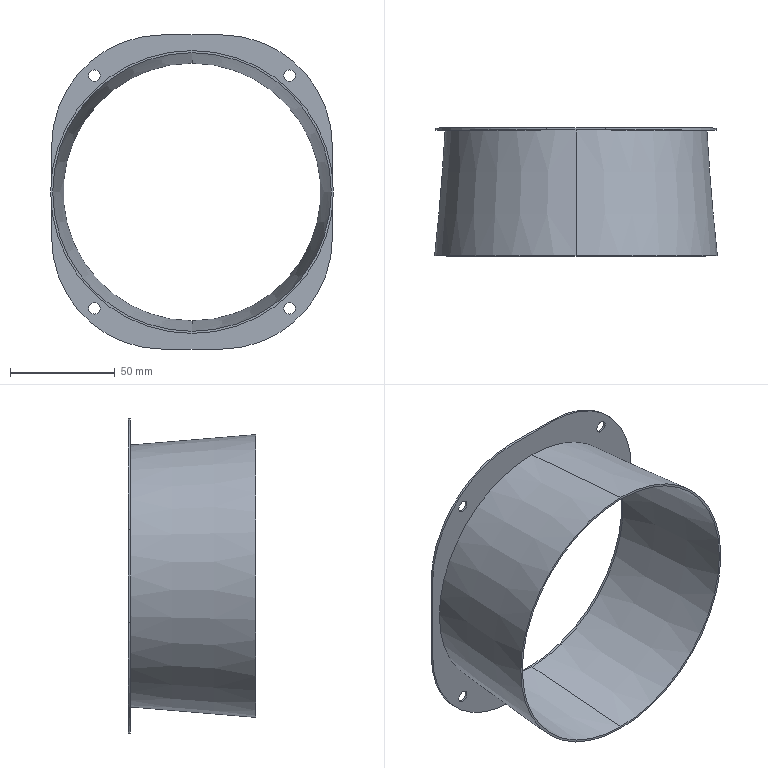Part | SolidWorks | features BaseBody 2 | 2 solids | 26 faces | box 135 x 61 x 150 mm | volume 30112 mm3 | cylinder 14 | plane 8 | cone 4 | commonest cylinder face diameters 5.5 x8 106 x4 122.993 x2
STEP:
#1=CARTESIAN_POINT('',(0.,0.,61.497));
#2=VERTEX_POINT('',#1);
#3=CARTESIAN_POINT('',(0.,-60.,66.497));
#4=VERTEX_POINT('',#3);
#5=CARTESIAN_POINT('',(0.,-0.08305,61.503));
#6=DIRECTION('',(0.,-0.9965,0.08305));
#7=VECTOR('',#6,1000.);
#8=LINE('',#5,#7);
#9=EDGE_CURVE('',#2,#4,#8,.T.);
#10=ORIENTED_EDGE('',*,*,#9,.F.);
#11=CARTESIAN_POINT('',(0.,0.,-61.497));
#12=VERTEX_POINT('',#11);
#13=CARTESIAN_POINT('',(0.,0.,0.));
#14=DIRECTION('',(0.,1.,0.));
#15=DIRECTION('',(0.,0.,1.));
#16=AXIS2_PLACEMENT_3D('',#13,#14,#15);
#17=CIRCLE('',#16,61.497);
#18=EDGE_CURVE('',#2,#12,#17,.T.);
#19=ORIENTED_EDGE('',*,*,#18,.T.);
#20=CARTESIAN_POINT('',(0.,-60.,-66.497));
#21=VERTEX_POINT('',#20);
#22=CARTESIAN_POINT('',(0.,-0.08305,-61.503));
#23=DIRECTION('',(0.,-0.9965,-0.08305));
#24=VECTOR('',#23,1000.);
#25=LINE('',#22,#24);
#26=EDGE_CURVE('',#12,#21,#25,.T.);
#27=ORIENTED_EDGE('',*,*,#26,.T.);
#28=CARTESIAN_POINT('',(0.,-60.,0.));
#29=DIRECTION('',(0.,1.,0.));
#30=DIRECTION('',(0.,0.,1.));
#31=AXIS2_PLACEMENT_3D('',#28,#29,#30);
#32=CIRCLE('',#31,66.497);
#33=EDGE_CURVE('',#4,#21,#32,.T.);
#34=ORIENTED_EDGE('',*,*,#33,.F.);
#35=EDGE_LOOP('',(#10,#19,#27,#34));
#36=FACE_OUTER_BOUND('',#35,.T.);
#37=CARTESIAN_POINT('',(0.,-0.08305,0.));
#38=DIRECTION('',(0.,-1.,0.));
#39=DIRECTION('',(0.,0.,-1.));
#40=AXIS2_PLACEMENT_3D('',#37,#38,#39);
#41=CONICAL_SURFACE('',#40,61.503,0.08314);
#42=ADVANCED_FACE('',(#36),#41,.F.);
#43=CARTESIAN_POINT('',(0.,0.,62.5));
#44=VERTEX_POINT('',#43);
#45=CARTESIAN_POINT('',(0.,-60.,67.5));
#46=VERTEX_POINT('',#45);
#47=CARTESIAN_POINT('',(0.,0.,62.5));
#48=DIRECTION('',(0.,-0.9965,0.08305));
#49=VECTOR('',#48,1000.);
#50=LINE('',#47,#49);
#51=EDGE_CURVE('',#44,#46,#50,.T.);
#52=ORIENTED_EDGE('',*,*,#51,.F.);
#53=CARTESIAN_POINT('',(0.,0.,-62.5));
#54=VERTEX_POINT('',#53);
#55=CARTESIAN_POINT('',(0.,0.,0.));
#56=DIRECTION('',(0.,1.,0.));
#57=DIRECTION('',(0.,0.,1.));
#58=AXIS2_PLACEMENT_3D('',#55,#56,#57);
#59=CIRCLE('',#58,62.5);
#60=EDGE_CURVE('',#54,#44,#59,.T.);
#61=ORIENTED_EDGE('',*,*,#60,.F.);
#62=CARTESIAN_POINT('',(0.,-60.,-67.5));
#63=VERTEX_POINT('',#62);
#64=CARTESIAN_POINT('',(0.,0.,-62.5));
#65=DIRECTION('',(0.,-0.9965,-0.08305));
#66=VECTOR('',#65,1000.);
#67=LINE('',#64,#66);
#68=EDGE_CURVE('',#54,#63,#67,.T.);
#69=ORIENTED_EDGE('',*,*,#68,.T.);
#70=CARTESIAN_POINT('',(0.,-60.,0.));
#71=DIRECTION('',(0.,1.,0.));
#72=DIRECTION('',(0.,0.,1.));
#73=AXIS2_PLACEMENT_3D('',#70,#71,#72);
#74=CIRCLE('',#73,67.5);
#75=EDGE_CURVE('',#63,#46,#74,.T.);
#76=ORIENTED_EDGE('',*,*,#75,.T.);
#77=EDGE_LOOP('',(#52,#61,#69,#76));
#78=FACE_OUTER_BOUND('',#77,.T.);
#79=CARTESIAN_POINT('',(0.,0.,0.));
#80=DIRECTION('',(0.,-1.,0.));
#81=DIRECTION('',(0.,0.,-1.));
#82=AXIS2_PLACEMENT_3D('',#79,#80,#81);
#83=CONICAL_SURFACE('',#82,62.5,0.08314);
#84=ADVANCED_FACE('',(#78),#83,.T.);
#85=CARTESIAN_POINT('',(0.,0.,0.));
#86=DIRECTION('',(0.,1.,0.));
#87=DIRECTION('',(0.,0.,1.));
#88=AXIS2_PLACEMENT_3D('',#85,#86,#87);
#89=CIRCLE('',#88,61.497);
#90=EDGE_CURVE('',#12,#2,#89,.T.);
#91=ORIENTED_EDGE('',*,*,#90,.F.);
#92=ORIENTED_EDGE('',*,*,#18,.F.);
#93=EDGE_LOOP('',(#91,#92));
#94=FACE_BOUND('',#93,.T.);
#95=ORIENTED_EDGE('',*,*,#60,.T.);
#96=CARTESIAN_POINT('',(0.,0.,0.));
#97=DIRECTION('',(0.,1.,0.));
#98=DIRECTION('',(0.,0.,1.));
#99=AXIS2_PLACEMENT_3D('',#96,#97,#98);
#100=CIRCLE('',#99,62.5);
#101=EDGE_CURVE('',#44,#54,#100,.T.);
#102=ORIENTED_EDGE('',*,*,#101,.T.);
#103=EDGE_LOOP('',(#95,#102));
#104=FACE_OUTER_BOUND('',#103,.T.);
#105=CARTESIAN_POINT('',(0.,0.,0.));
#106=DIRECTION('',(0.,1.,0.));
#107=DIRECTION('',(1.,0.,0.));
#108=AXIS2_PLACEMENT_3D('',#105,#106,#107);
#109=PLANE('',#108);
#110=ADVANCED_FACE('',(#94,#104),#109,.T.);
#111=CARTESIAN_POINT('',(0.,-60.,0.));
#112=DIRECTION('',(0.,1.,0.));
#113=DIRECTION('',(0.,0.,1.));
#114=AXIS2_PLACEMENT_3D('',#111,#112,#113);
#115=CIRCLE('',#114,66.497);
#116=EDGE_CURVE('',#21,#4,#115,.T.);
#117=ORIENTED_EDGE('',*,*,#116,.T.);
#118=ORIENTED_EDGE('',*,*,#33,.T.);
#119=EDGE_LOOP('',(#117,#118));
#120=FACE_BOUND('',#119,.T.);
#121=ORIENTED_EDGE('',*,*,#75,.F.);
#122=CARTESIAN_POINT('',(0.,-60.,0.));
#123=DIRECTION('',(0.,1.,0.));
#124=DIRECTION('',(0.,0.,1.));
#125=AXIS2_PLACEMENT_3D('',#122,#123,#124);
#126=CIRCLE('',#125,67.5);
#127=EDGE_CURVE('',#46,#63,#126,.T.);
#128=ORIENTED_EDGE('',*,*,#127,.F.);
#129=EDGE_LOOP('',(#121,#128));
#130=FACE_OUTER_BOUND('',#129,.T.);
#131=CARTESIAN_POINT('',(0.,-60.,0.));
#132=DIRECTION('',(0.,1.,0.));
#133=DIRECTION('',(1.,0.,0.));
#134=AXIS2_PLACEMENT_3D('',#131,#132,#133);
#135=PLANE('',#134);
#136=ADVANCED_FACE('',(#120,#130),#135,.F.);
#137=ORIENTED_EDGE('',*,*,#101,.F.);
#138=ORIENTED_EDGE('',*,*,#51,.T.);
#139=ORIENTED_EDGE('',*,*,#127,.T.);
#140=ORIENTED_EDGE('',*,*,#68,.F.);
#141=EDGE_LOOP('',(#137,#138,#139,#140));
#142=FACE_OUTER_BOUND('',#141,.T.);
#143=CARTESIAN_POINT('',(0.,0.,0.));
#144=DIRECTION('',(0.,-1.,0.));
#145=DIRECTION('',(0.,0.,-1.));
#146=AXIS2_PLACEMENT_3D('',#143,#144,#145);
#147=CONICAL_SURFACE('',#146,62.5,0.08314);
#148=ADVANCED_FACE('',(#142),#147,.T.);
#149=ORIENTED_EDGE('',*,*,#90,.T.);
#150=ORIENTED_EDGE('',*,*,#9,.T.);
#151=ORIENTED_EDGE('',*,*,#116,.F.);
#152=ORIENTED_EDGE('',*,*,#26,.F.);
#153=EDGE_LOOP('',(#149,#150,#151,#152));
#154=FACE_OUTER_BOUND('',#153,.T.);
#155=CARTESIAN_POINT('',(0.,-0.08305,0.));
#156=DIRECTION('',(0.,-1.,0.));
#157=DIRECTION('',(0.,0.,-1.));
#158=AXIS2_PLACEMENT_3D('',#155,#156,#157);
#159=CONICAL_SURFACE('',#158,61.503,0.08314);
#160=ADVANCED_FACE('',(#154),#159,.F.);
#161=CLOSED_SHELL('',(#42,#84,#110,#136,#148,#160));
#162=MANIFOLD_SOLID_BREP('',#161);
#163=CARTESIAN_POINT('',(0.,1.,61.497));
#164=VERTEX_POINT('',#163);
#165=CARTESIAN_POINT('',(0.,0.,61.497));
#166=VERTEX_POINT('',#165);
#167=CARTESIAN_POINT('',(0.,174.938,61.497));
#168=DIRECTION('',(0.,-1.,0.));
#169=VECTOR('',#168,1000.);
#170=LINE('',#167,#169);
#171=EDGE_CURVE('',#164,#166,#170,.T.);
#172=ORIENTED_EDGE('',*,*,#171,.F.);
#173=CARTESIAN_POINT('',(0.,1.,-61.497));
#174=VERTEX_POINT('',#173);
#175=CARTESIAN_POINT('',(0.,1.,0.));
#176=DIRECTION('',(0.,-1.,0.));
#177=DIRECTION('',(0.,0.,1.));
#178=AXIS2_PLACEMENT_3D('',#175,#176,#177);
#179=CIRCLE('',#178,61.497);
#180=EDGE_CURVE('',#174,#164,#179,.T.);
#181=ORIENTED_EDGE('',*,*,#180,.F.);
#182=CARTESIAN_POINT('',(0.,0.,-61.497));
#183=VERTEX_POINT('',#182);
#184=CARTESIAN_POINT('',(0.,174.938,-61.497));
#185=DIRECTION('',(0.,-1.,0.));
#186=VECTOR('',#185,1000.);
#187=LINE('',#184,#186);
#188=EDGE_CURVE('',#174,#183,#187,.T.);
#189=ORIENTED_EDGE('',*,*,#188,.T.);
#190=CARTESIAN_POINT('',(0.,0.,0.));
#191=DIRECTION('',(0.,-1.,0.));
#192=DIRECTION('',(0.,0.,-1.));
#193=AXIS2_PLACEMENT_3D('',#190,#191,#192);
#194=CIRCLE('',#193,61.497);
#195=EDGE_CURVE('',#183,#166,#194,.T.);
#196=ORIENTED_EDGE('',*,*,#195,.T.);
#197=EDGE_LOOP('',(#172,#181,#189,#196));
#198=FACE_OUTER_BOUND('',#197,.T.);
#199=CARTESIAN_POINT('',(0.,174.938,0.));
#200=DIRECTION('',(0.,-1.,0.));
#201=DIRECTION('',(0.,0.,-1.));
#202=AXIS2_PLACEMENT_3D('',#199,#200,#201);
#203=CYLINDRICAL_SURFACE('',#202,61.497);
#204=ADVANCED_FACE('',(#198),#203,.F.);
#205=CARTESIAN_POINT('',(46.602,0.,-58.288));
#206=VERTEX_POINT('',#205);
#207=CARTESIAN_POINT('',(46.602,1.,-58.288));
#208=VERTEX_POINT('',#207);
#209=CARTESIAN_POINT('',(46.602,1.,-58.288));
#210=DIRECTION('',(0.,1.,0.));
#211=VECTOR('',#210,1000.);
#212=LINE('',#209,#211);
#213=EDGE_CURVE('',#206,#208,#212,.T.);
#214=ORIENTED_EDGE('',*,*,#213,.F.);
#215=CARTESIAN_POINT('',(46.602,0.,-52.788));
#216=VERTEX_POINT('',#215);
#217=CARTESIAN_POINT('',(46.602,0.,-55.538));
#218=DIRECTION('',(0.,1.,0.));
#219=DIRECTION('',(0.,0.,1.));
#220=AXIS2_PLACEMENT_3D('',#217,#218,#219);
#221=CIRCLE('',#220,2.75);
#222=EDGE_CURVE('',#216,#206,#221,.T.);
#223=ORIENTED_EDGE('',*,*,#222,.F.);
#224=CARTESIAN_POINT('',(46.602,1.,-52.788));
#225=VERTEX_POINT('',#224);
#226=CARTESIAN_POINT('',(46.602,1.,-52.788));
#227=DIRECTION('',(0.,1.,0.));
#228=VECTOR('',#227,1000.);
#229=LINE('',#226,#228);
#230=EDGE_CURVE('',#216,#225,#229,.T.);
#231=ORIENTED_EDGE('',*,*,#230,.T.);
#232=CARTESIAN_POINT('',(46.602,1.,-55.538));
#233=DIRECTION('',(0.,1.,0.));
#234=DIRECTION('',(0.,0.,1.));
#235=AXIS2_PLACEMENT_3D('',#232,#233,#234);
#236=CIRCLE('',#235,2.75);
#237=EDGE_CURVE('',#225,#208,#236,.T.);
#238=ORIENTED_EDGE('',*,*,#237,.T.);
#239=EDGE_LOOP('',(#214,#223,#231,#238));
#240=FACE_OUTER_BOUND('',#239,.T.);
#241=CARTESIAN_POINT('',(46.602,1.,-55.538));
#242=DIRECTION('',(0.,1.,0.));
#243=DIRECTION('',(0.,0.,1.));
#244=AXIS2_PLACEMENT_3D('',#241,#242,#243);
#245=CYLINDRICAL_SURFACE('',#244,2.75);
#246=ADVANCED_FACE('',(#240),#245,.F.);
#247=CARTESIAN_POINT('',(46.602,0.,52.788));
#248=VERTEX_POINT('',#247);
#249=CARTESIAN_POINT('',(46.602,1.,52.788));
#250=VERTEX_POINT('',#249);
#251=CARTESIAN_POINT('',(46.602,1.,52.788));
#252=DIRECTION('',(0.,1.,0.));
#253=VECTOR('',#252,1000.);
#254=LINE('',#251,#253);
#255=EDGE_CURVE('',#248,#250,#254,.T.);
#256=ORIENTED_EDGE('',*,*,#255,.F.);
#257=CARTESIAN_POINT('',(46.602,0.,58.288));
#258=VERTEX_POINT('',#257);
#259=CARTESIAN_POINT('',(46.602,0.,55.538));
#260=DIRECTION('',(0.,1.,0.));
#261=DIRECTION('',(0.,0.,1.));
#262=AXIS2_PLACEMENT_3D('',#259,#260,#261);
#263=CIRCLE('',#262,2.75);
#264=EDGE_CURVE('',#258,#248,#263,.T.);
#265=ORIENTED_EDGE('',*,*,#264,.F.);
#266=CARTESIAN_POINT('',(46.602,1.,58.288));
#267=VERTEX_POINT('',#266);
#268=CARTESIAN_POINT('',(46.602,1.,58.288));
#269=DIRECTION('',(0.,1.,0.));
#270=VECTOR('',#269,1000.);
#271=LINE('',#268,#270);
#272=EDGE_CURVE('',#258,#267,#271,.T.);
#273=ORIENTED_EDGE('',*,*,#272,.T.);
#274=CARTESIAN_POINT('',(46.602,1.,55.538));
#275=DIRECTION('',(0.,1.,0.));
#276=DIRECTION('',(0.,0.,1.));
#277=AXIS2_PLACEMENT_3D('',#274,#275,#276);
#278=CIRCLE('',#277,2.75);
#279=EDGE_CURVE('',#267,#250,#278,.T.);
#280=ORIENTED_EDGE('',*,*,#279,.T.);
#281=EDGE_LOOP('',(#256,#265,#273,#280));
#282=FACE_OUTER_BOUND('',#281,.T.);
#283=CARTESIAN_POINT('',(46.602,1.,55.538));
#284=DIRECTION('',(0.,1.,0.));
#285=DIRECTION('',(0.,0.,1.));
#286=AXIS2_PLACEMENT_3D('',#283,#284,#285);
#287=CYLINDRICAL_SURFACE('',#286,2.75);
#288=ADVANCED_FACE('',(#282),#287,.F.);
#289=CARTESIAN_POINT('',(-46.602,0.,52.788));
#290=VERTEX_POINT('',#289);
#291=CARTESIAN_POINT('',(-46.602,1.,52.788));
#292=VERTEX_POINT('',#291);
#293=CARTESIAN_POINT('',(-46.602,1.,52.788));
#294=DIRECTION('',(0.,1.,0.));
#295=VECTOR('',#294,1000.);
#296=LINE('',#293,#295);
#297=EDGE_CURVE('',#290,#292,#296,.T.);
#298=ORIENTED_EDGE('',*,*,#297,.F.);
#299=CARTESIAN_POINT('',(-46.602,0.,58.288));
#300=VERTEX_POINT('',#299);
#301=CARTESIAN_POINT('',(-46.602,0.,55.538));
#302=DIRECTION('',(0.,1.,0.));
#303=DIRECTION('',(0.,0.,1.));
#304=AXIS2_PLACEMENT_3D('',#301,#302,#303);
#305=CIRCLE('',#304,2.75);
#306=EDGE_CURVE('',#300,#290,#305,.T.);
#307=ORIENTED_EDGE('',*,*,#306,.F.);
#308=CARTESIAN_POINT('',(-46.602,1.,58.288));
#309=VERTEX_POINT('',#308);
#310=CARTESIAN_POINT('',(-46.602,1.,58.288));
#311=DIRECTION('',(0.,1.,0.));
#312=VECTOR('',#311,1000.);
#313=LINE('',#310,#312);
#314=EDGE_CURVE('',#300,#309,#313,.T.);
#315=ORIENTED_EDGE('',*,*,#314,.T.);
#316=CARTESIAN_POINT('',(-46.602,1.,55.538));
#317=DIRECTION('',(0.,1.,0.));
#318=DIRECTION('',(0.,0.,1.));
#319=AXIS2_PLACEMENT_3D('',#316,#317,#318);
#320=CIRCLE('',#319,2.75);
#321=EDGE_CURVE('',#309,#292,#320,.T.);
#322=ORIENTED_EDGE('',*,*,#321,.T.);
#323=EDGE_LOOP('',(#298,#307,#315,#322));
#324=FACE_OUTER_BOUND('',#323,.T.);
#325=CARTESIAN_POINT('',(-46.602,1.,55.538));
#326=DIRECTION('',(0.,1.,0.));
#327=DIRECTION('',(0.,0.,1.));
#328=AXIS2_PLACEMENT_3D('',#325,#326,#327);
#329=CYLINDRICAL_SURFACE('',#328,2.75);
#330=ADVANCED_FACE('',(#324),#329,.F.);
#331=CARTESIAN_POINT('',(-46.602,0.,-58.288));
#332=VERTEX_POINT('',#331);
#333=CARTESIAN_POINT('',(-46.602,1.,-58.288));
#334=VERTEX_POINT('',#333);
#335=CARTESIAN_POINT('',(-46.602,1.,-58.288));
#336=DIRECTION('',(0.,1.,0.));
#337=VECTOR('',#336,1000.);
#338=LINE('',#335,#337);
#339=EDGE_CURVE('',#332,#334,#338,.T.);
#340=ORIENTED_EDGE('',*,*,#339,.F.);
#341=CARTESIAN_POINT('',(-46.602,0.,-52.788));
#342=VERTEX_POINT('',#341);
#343=CARTESIAN_POINT('',(-46.602,0.,-55.538));
#344=DIRECTION('',(0.,1.,0.));
#345=DIRECTION('',(0.,0.,1.));
#346=AXIS2_PLACEMENT_3D('',#343,#344,#345);
#347=CIRCLE('',#346,2.75);
#348=EDGE_CURVE('',#342,#332,#347,.T.);
#349=ORIENTED_EDGE('',*,*,#348,.F.);
#350=CARTESIAN_POINT('',(-46.602,1.,-52.788));
#351=VERTEX_POINT('',#350);
#352=CARTESIAN_POINT('',(-46.602,1.,-52.788));
#353=DIRECTION('',(0.,1.,0.));
#354=VECTOR('',#353,1000.);
#355=LINE('',#352,#354);
#356=EDGE_CURVE('',#342,#351,#355,.T.);
#357=ORIENTED_EDGE('',*,*,#356,.T.);
#358=CARTESIAN_POINT('',(-46.602,1.,-55.538));
#359=DIRECTION('',(0.,1.,0.));
#360=DIRECTION('',(0.,0.,1.));
#361=AXIS2_PLACEMENT_3D('',#358,#359,#360);
#362=CIRCLE('',#361,2.75);
#363=EDGE_CURVE('',#351,#334,#362,.T.);
#364=ORIENTED_EDGE('',*,*,#363,.T.);
#365=EDGE_LOOP('',(#340,#349,#357,#364));
#366=FACE_OUTER_BOUND('',#365,.T.);
#367=CARTESIAN_POINT('',(-46.602,1.,-55.538));
#368=DIRECTION('',(0.,1.,0.));
#369=DIRECTION('',(0.,0.,1.));
#370=AXIS2_PLACEMENT_3D('',#367,#368,#369);
#371=CYLINDRICAL_SURFACE('',#370,2.75);
#372=ADVANCED_FACE('',(#366),#371,.F.);
#373=ORIENTED_EDGE('',*,*,#348,.T.);
#374=CARTESIAN_POINT('',(-46.602,0.,-55.538));
#375=DIRECTION('',(0.,1.,0.));
#376=DIRECTION('',(0.,0.,1.));
#377=AXIS2_PLACEMENT_3D('',#374,#375,#376);
#378=CIRCLE('',#377,2.75);
#379=EDGE_CURVE('',#332,#342,#378,.T.);
#380=ORIENTED_EDGE('',*,*,#379,.T.);
#381=EDGE_LOOP('',(#373,#380));
#382=FACE_BOUND('',#381,.T.);
#383=ORIENTED_EDGE('',*,*,#306,.T.);
#384=CARTESIAN_POINT('',(-46.602,0.,55.538));
#385=DIRECTION('',(0.,1.,0.));
#386=DIRECTION('',(0.,0.,1.));
#387=AXIS2_PLACEMENT_3D('',#384,#385,#386);
#388=CIRCLE('',#387,2.75);
#389=EDGE_CURVE('',#290,#300,#388,.T.);
#390=ORIENTED_EDGE('',*,*,#389,.T.);
#391=EDGE_LOOP('',(#383,#390));
#392=FACE_BOUND('',#391,.T.);
#393=ORIENTED_EDGE('',*,*,#264,.T.);
#394=CARTESIAN_POINT('',(46.602,0.,55.538));
#395=DIRECTION('',(0.,1.,0.));
#396=DIRECTION('',(0.,0.,1.));
#397=AXIS2_PLACEMENT_3D('',#394,#395,#396);
#398=CIRCLE('',#397,2.75);
#399=EDGE_CURVE('',#248,#258,#398,.T.);
#400=ORIENTED_EDGE('',*,*,#399,.T.);
#401=EDGE_LOOP('',(#393,#400));
#402=FACE_BOUND('',#401,.T.);
#403=ORIENTED_EDGE('',*,*,#222,.T.);
#404=CARTESIAN_POINT('',(46.602,0.,-55.538));
#405=DIRECTION('',(0.,1.,0.));
#406=DIRECTION('',(0.,0.,1.));
#407=AXIS2_PLACEMENT_3D('',#404,#405,#406);
#408=CIRCLE('',#407,2.75);
#409=EDGE_CURVE('',#206,#216,#408,.T.);
#410=ORIENTED_EDGE('',*,*,#409,.T.);
#411=EDGE_LOOP('',(#403,#410));
#412=FACE_BOUND('',#411,.T.);
#413=ORIENTED_EDGE('',*,*,#195,.F.);
#414=CARTESIAN_POINT('',(0.,0.,0.));
#415=DIRECTION('',(0.,-1.,0.));
#416=DIRECTION('',(0.,0.,-1.));
#417=AXIS2_PLACEMENT_3D('',#414,#415,#416);
#418=CIRCLE('',#417,61.497);
#419=EDGE_CURVE('',#166,#183,#418,.T.);
#420=ORIENTED_EDGE('',*,*,#419,.F.);
#421=EDGE_LOOP('',(#413,#420));
#422=FACE_BOUND('',#421,.T.);
#423=CARTESIAN_POINT('',(14.,0.,75.));
#424=VERTEX_POINT('',#423);
#425=CARTESIAN_POINT('',(67.,0.,22.));
#426=VERTEX_POINT('',#425);
#427=CARTESIAN_POINT('',(14.,0.,22.));
#428=DIRECTION('',(0.,1.,0.));
#429=DIRECTION('',(0.,0.,1.));
#430=AXIS2_PLACEMENT_3D('',#427,#428,#429);
#431=CIRCLE('',#430,53.);
#432=EDGE_CURVE('',#424,#426,#431,.T.);
#433=ORIENTED_EDGE('',*,*,#432,.F.);
#434=CARTESIAN_POINT('',(-14.,0.,75.));
#435=VERTEX_POINT('',#434);
#436=CARTESIAN_POINT('',(14.,0.,75.));
#437=DIRECTION('',(1.,0.,0.));
#438=VECTOR('',#437,1000.);
#439=LINE('',#436,#438);
#440=EDGE_CURVE('',#435,#424,#439,.T.);
#441=ORIENTED_EDGE('',*,*,#440,.F.);
#442=CARTESIAN_POINT('',(-67.,0.,22.));
#443=VERTEX_POINT('',#442);
#444=CARTESIAN_POINT('',(-14.,0.,22.));
#445=DIRECTION('',(0.,1.,0.));
#446=DIRECTION('',(0.,0.,-1.));
#447=AXIS2_PLACEMENT_3D('',#444,#445,#446);
#448=CIRCLE('',#447,53.);
#449=EDGE_CURVE('',#443,#435,#448,.T.);
#450=ORIENTED_EDGE('',*,*,#449,.F.);
#451=CARTESIAN_POINT('',(-67.,0.,-22.));
#452=VERTEX_POINT('',#451);
#453=CARTESIAN_POINT('',(-67.,0.,22.));
#454=DIRECTION('',(0.,0.,1.));
#455=VECTOR('',#454,1000.);
#456=LINE('',#453,#455);
#457=EDGE_CURVE('',#452,#443,#456,.T.);
#458=ORIENTED_EDGE('',*,*,#457,.F.);
#459=CARTESIAN_POINT('',(-14.,0.,-75.));
#460=VERTEX_POINT('',#459);
#461=CARTESIAN_POINT('',(-14.,0.,-22.));
#462=DIRECTION('',(0.,1.,0.));
#463=DIRECTION('',(0.,0.,1.));
#464=AXIS2_PLACEMENT_3D('',#461,#462,#463);
#465=CIRCLE('',#464,53.);
#466=EDGE_CURVE('',#460,#452,#465,.T.);
#467=ORIENTED_EDGE('',*,*,#466,.F.);
#468=CARTESIAN_POINT('',(14.,0.,-75.));
#469=VERTEX_POINT('',#468);
#470=CARTESIAN_POINT('',(14.,0.,-75.));
#471=DIRECTION('',(-1.,0.,0.));
#472=VECTOR('',#471,1000.);
#473=LINE('',#470,#472);
#474=EDGE_CURVE('',#469,#460,#473,.T.);
#475=ORIENTED_EDGE('',*,*,#474,.F.);
#476=CARTESIAN_POINT('',(67.,0.,-22.));
#477=VERTEX_POINT('',#476);
#478=CARTESIAN_POINT('',(14.,0.,-22.));
#479=DIRECTION('',(0.,1.,0.));
#480=DIRECTION('',(0.,0.,1.));
#481=AXIS2_PLACEMENT_3D('',#478,#479,#480);
#482=CIRCLE('',#481,53.);
#483=EDGE_CURVE('',#477,#469,#482,.T.);
#484=ORIENTED_EDGE('',*,*,#483,.F.);
#485=CARTESIAN_POINT('',(67.,0.,22.));
#486=DIRECTION('',(0.,0.,-1.));
#487=VECTOR('',#486,1000.);
#488=LINE('',#485,#487);
#489=EDGE_CURVE('',#426,#477,#488,.T.);
#490=ORIENTED_EDGE('',*,*,#489,.F.);
#491=EDGE_LOOP('',(#433,#441,#450,#458,#467,#475,#484,#490));
#492=FACE_OUTER_BOUND('',#491,.T.);
#493=CARTESIAN_POINT('',(14.,0.,22.));
#494=DIRECTION('',(0.,1.,0.));
#495=DIRECTION('',(1.,0.,0.));
#496=AXIS2_PLACEMENT_3D('',#493,#494,#495);
#497=PLANE('',#496);
#498=ADVANCED_FACE('',(#382,#392,#402,#412,#422,#492),#497,.F.);
#499=ORIENTED_EDGE('',*,*,#363,.F.);
#500=CARTESIAN_POINT('',(-46.602,1.,-55.538));
#501=DIRECTION('',(0.,1.,0.));
#502=DIRECTION('',(0.,0.,1.));
#503=AXIS2_PLACEMENT_3D('',#500,#501,#502);
#504=CIRCLE('',#503,2.75);
#505=EDGE_CURVE('',#334,#351,#504,.T.);
#506=ORIENTED_EDGE('',*,*,#505,.F.);
#507=EDGE_LOOP('',(#499,#506));
#508=FACE_BOUND('',#507,.T.);
#509=ORIENTED_EDGE('',*,*,#321,.F.);
#510=CARTESIAN_POINT('',(-46.602,1.,55.538));
#511=DIRECTION('',(0.,1.,0.));
#512=DIRECTION('',(0.,0.,1.));
#513=AXIS2_PLACEMENT_3D('',#510,#511,#512);
#514=CIRCLE('',#513,2.75);
#515=EDGE_CURVE('',#292,#309,#514,.T.);
#516=ORIENTED_EDGE('',*,*,#515,.F.);
#517=EDGE_LOOP('',(#509,#516));
#518=FACE_BOUND('',#517,.T.);
#519=ORIENTED_EDGE('',*,*,#279,.F.);
#520=CARTESIAN_POINT('',(46.602,1.,55.538));
#521=DIRECTION('',(0.,1.,0.));
#522=DIRECTION('',(0.,0.,1.));
#523=AXIS2_PLACEMENT_3D('',#520,#521,#522);
#524=CIRCLE('',#523,2.75);
#525=EDGE_CURVE('',#250,#267,#524,.T.);
#526=ORIENTED_EDGE('',*,*,#525,.F.);
#527=EDGE_LOOP('',(#519,#526));
#528=FACE_BOUND('',#527,.T.);
#529=ORIENTED_EDGE('',*,*,#237,.F.);
#530=CARTESIAN_POINT('',(46.602,1.,-55.538));
#531=DIRECTION('',(0.,1.,0.));
#532=DIRECTION('',(0.,0.,1.));
#533=AXIS2_PLACEMENT_3D('',#530,#531,#532);
#534=CIRCLE('',#533,2.75);
#535=EDGE_CURVE('',#208,#225,#534,.T.);
#536=ORIENTED_EDGE('',*,*,#535,.F.);
#537=EDGE_LOOP('',(#529,#536));
#538=FACE_BOUND('',#537,.T.);
#539=ORIENTED_EDGE('',*,*,#180,.T.);
#540=CARTESIAN_POINT('',(0.,1.,0.));
#541=DIRECTION('',(0.,-1.,0.));
#542=DIRECTION('',(0.,0.,1.));
#543=AXIS2_PLACEMENT_3D('',#540,#541,#542);
#544=CIRCLE('',#543,61.497);
#545=EDGE_CURVE('',#164,#174,#544,.T.);
#546=ORIENTED_EDGE('',*,*,#545,.T.);
#547=EDGE_LOOP('',(#539,#546));
#548=FACE_BOUND('',#547,.T.);
#549=CARTESIAN_POINT('',(14.,1.,75.));
#550=VERTEX_POINT('',#549);
#551=CARTESIAN_POINT('',(67.,1.,22.));
#552=VERTEX_POINT('',#551);
#553=CARTESIAN_POINT('',(14.,1.,22.));
#554=DIRECTION('',(0.,1.,0.));
#555=DIRECTION('',(0.,0.,1.));
#556=AXIS2_PLACEMENT_3D('',#553,#554,#555);
#557=CIRCLE('',#556,53.);
#558=EDGE_CURVE('',#550,#552,#557,.T.);
#559=ORIENTED_EDGE('',*,*,#558,.T.);
#560=CARTESIAN_POINT('',(67.,1.,-22.));
#561=VERTEX_POINT('',#560);
#562=CARTESIAN_POINT('',(67.,1.,22.));
#563=DIRECTION('',(0.,0.,-1.));
#564=VECTOR('',#563,1000.);
#565=LINE('',#562,#564);
#566=EDGE_CURVE('',#552,#561,#565,.T.);
#567=ORIENTED_EDGE('',*,*,#566,.T.);
#568=CARTESIAN_POINT('',(14.,1.,-75.));
#569=VERTEX_POINT('',#568);
#570=CARTESIAN_POINT('',(14.,1.,-22.));
#571=DIRECTION('',(0.,1.,0.));
#572=DIRECTION('',(0.,0.,1.));
#573=AXIS2_PLACEMENT_3D('',#570,#571,#572);
#574=CIRCLE('',#573,53.);
#575=EDGE_CURVE('',#561,#569,#574,.T.);
#576=ORIENTED_EDGE('',*,*,#575,.T.);
#577=CARTESIAN_POINT('',(-14.,1.,-75.));
#578=VERTEX_POINT('',#577);
#579=CARTESIAN_POINT('',(14.,1.,-75.));
#580=DIRECTION('',(-1.,0.,0.));
#581=VECTOR('',#580,1000.);
#582=LINE('',#579,#581);
#583=EDGE_CURVE('',#569,#578,#582,.T.);
#584=ORIENTED_EDGE('',*,*,#583,.T.);
#585=CARTESIAN_POINT('',(-67.,1.,-22.));
#586=VERTEX_POINT('',#585);
#587=CARTESIAN_POINT('',(-14.,1.,-22.));
#588=DIRECTION('',(0.,1.,0.));
#589=DIRECTION('',(0.,0.,1.));
#590=AXIS2_PLACEMENT_3D('',#587,#588,#589);
#591=CIRCLE('',#590,53.);
#592=EDGE_CURVE('',#578,#586,#591,.T.);
#593=ORIENTED_EDGE('',*,*,#592,.T.);
#594=CARTESIAN_POINT('',(-67.,1.,22.));
#595=VERTEX_POINT('',#594);
#596=CARTESIAN_POINT('',(-67.,1.,22.));
#597=DIRECTION('',(0.,0.,1.));
#598=VECTOR('',#597,1000.);
#599=LINE('',#596,#598);
#600=EDGE_CURVE('',#586,#595,#599,.T.);
#601=ORIENTED_EDGE('',*,*,#600,.T.);
#602=CARTESIAN_POINT('',(-14.,1.,75.));
#603=VERTEX_POINT('',#602);
#604=CARTESIAN_POINT('',(-14.,1.,22.));
#605=DIRECTION('',(0.,1.,0.));
#606=DIRECTION('',(0.,0.,-1.));
#607=AXIS2_PLACEMENT_3D('',#604,#605,#606);
#608=CIRCLE('',#607,53.);
#609=EDGE_CURVE('',#595,#603,#608,.T.);
#610=ORIENTED_EDGE('',*,*,#609,.T.);
#611=CARTESIAN_POINT('',(14.,1.,75.));
#612=DIRECTION('',(1.,0.,0.));
#613=VECTOR('',#612,1000.);
#614=LINE('',#611,#613);
#615=EDGE_CURVE('',#603,#550,#614,.T.);
#616=ORIENTED_EDGE('',*,*,#615,.T.);
#617=EDGE_LOOP('',(#559,#567,#576,#584,#593,#601,#610,#616));
#618=FACE_OUTER_BOUND('',#617,.T.);
#619=CARTESIAN_POINT('',(14.,1.,22.));
#620=DIRECTION('',(0.,1.,0.));
#621=DIRECTION('',(1.,0.,0.));
#622=AXIS2_PLACEMENT_3D('',#619,#620,#621);
#623=PLANE('',#622);
#624=ADVANCED_FACE('',(#508,#518,#528,#538,#548,#618),#623,.T.);
#625=ORIENTED_EDGE('',*,*,#440,.T.);
#626=CARTESIAN_POINT('',(14.,1.,75.));
#627=DIRECTION('',(0.,-1.,0.));
#628=VECTOR('',#627,1000.);
#629=LINE('',#626,#628);
#630=EDGE_CURVE('',#550,#424,#629,.T.);
#631=ORIENTED_EDGE('',*,*,#630,.F.);
#632=ORIENTED_EDGE('',*,*,#615,.F.);
#633=CARTESIAN_POINT('',(-14.,1.,75.));
#634=DIRECTION('',(0.,-1.,0.));
#635=VECTOR('',#634,1000.);
#636=LINE('',#633,#635);
#637=EDGE_CURVE('',#603,#435,#636,.T.);
#638=ORIENTED_EDGE('',*,*,#637,.T.);
#639=EDGE_LOOP('',(#625,#631,#632,#638));
#640=FACE_OUTER_BOUND('',#639,.T.);
#641=CARTESIAN_POINT('',(14.,1.,75.));
#642=DIRECTION('',(0.,0.,-1.));
#643=DIRECTION('',(0.,-1.,0.));
#644=AXIS2_PLACEMENT_3D('',#641,#642,#643);
#645=PLANE('',#644);
#646=ADVANCED_FACE('',(#640),#645,.F.);
#647=ORIENTED_EDGE('',*,*,#449,.T.);
#648=ORIENTED_EDGE('',*,*,#637,.F.);
#649=ORIENTED_EDGE('',*,*,#609,.F.);
#650=CARTESIAN_POINT('',(-67.,1.,22.));
#651=DIRECTION('',(0.,-1.,0.));
#652=VECTOR('',#651,1000.);
#653=LINE('',#650,#652);
#654=EDGE_CURVE('',#595,#443,#653,.T.);
#655=ORIENTED_EDGE('',*,*,#654,.T.);
#656=EDGE_LOOP('',(#647,#648,#649,#655));
#657=FACE_OUTER_BOUND('',#656,.T.);
#658=CARTESIAN_POINT('',(-14.,1.,22.));
#659=DIRECTION('',(0.,-1.,0.));
#660=DIRECTION('',(0.,0.,-1.));
#661=AXIS2_PLACEMENT_3D('',#658,#659,#660);
#662=CYLINDRICAL_SURFACE('',#661,53.);
#663=ADVANCED_FACE('',(#657),#662,.T.);
#664=ORIENTED_EDGE('',*,*,#457,.T.);
#665=ORIENTED_EDGE('',*,*,#654,.F.);
#666=ORIENTED_EDGE('',*,*,#600,.F.);
#667=CARTESIAN_POINT('',(-67.,1.,-22.));
#668=DIRECTION('',(0.,-1.,0.));
#669=VECTOR('',#668,1000.);
#670=LINE('',#667,#669);
#671=EDGE_CURVE('',#586,#452,#670,.T.);
#672=ORIENTED_EDGE('',*,*,#671,.T.);
#673=EDGE_LOOP('',(#664,#665,#666,#672));
#674=FACE_OUTER_BOUND('',#673,.T.);
#675=CARTESIAN_POINT('',(-67.,1.,22.));
#676=DIRECTION('',(1.,0.,0.));
#677=DIRECTION('',(0.,1.,0.));
#678=AXIS2_PLACEMENT_3D('',#675,#676,#677);
#679=PLANE('',#678);
#680=ADVANCED_FACE('',(#674),#679,.F.);
#681=ORIENTED_EDGE('',*,*,#466,.T.);
#682=ORIENTED_EDGE('',*,*,#671,.F.);
#683=ORIENTED_EDGE('',*,*,#592,.F.);
#684=CARTESIAN_POINT('',(-14.,1.,-75.));
#685=DIRECTION('',(0.,-1.,0.));
#686=VECTOR('',#685,1000.);
#687=LINE('',#684,#686);
#688=EDGE_CURVE('',#578,#460,#687,.T.);
#689=ORIENTED_EDGE('',*,*,#688,.T.);
#690=EDGE_LOOP('',(#681,#682,#683,#689));
#691=FACE_OUTER_BOUND('',#690,.T.);
#692=CARTESIAN_POINT('',(-14.,1.,-22.));
#693=DIRECTION('',(0.,-1.,0.));
#694=DIRECTION('',(0.,0.,-1.));
#695=AXIS2_PLACEMENT_3D('',#692,#693,#694);
#696=CYLINDRICAL_SURFACE('',#695,53.);
#697=ADVANCED_FACE('',(#691),#696,.T.);
#698=ORIENTED_EDGE('',*,*,#474,.T.);
#699=ORIENTED_EDGE('',*,*,#688,.F.);
#700=ORIENTED_EDGE('',*,*,#583,.F.);
#701=CARTESIAN_POINT('',(14.,1.,-75.));
#702=DIRECTION('',(0.,-1.,0.));
#703=VECTOR('',#702,1000.);
#704=LINE('',#701,#703);
#705=EDGE_CURVE('',#569,#469,#704,.T.);
#706=ORIENTED_EDGE('',*,*,#705,.T.);
#707=EDGE_LOOP('',(#698,#699,#700,#706));
#708=FACE_OUTER_BOUND('',#707,.T.);
#709=CARTESIAN_POINT('',(14.,1.,-75.));
#710=DIRECTION('',(0.,0.,1.));
#711=DIRECTION('',(1.,0.,0.));
#712=AXIS2_PLACEMENT_3D('',#709,#710,#711);
#713=PLANE('',#712);
#714=ADVANCED_FACE('',(#708),#713,.F.);
#715=ORIENTED_EDGE('',*,*,#483,.T.);
#716=ORIENTED_EDGE('',*,*,#705,.F.);
#717=ORIENTED_EDGE('',*,*,#575,.F.);
#718=CARTESIAN_POINT('',(67.,1.,-22.));
#719=DIRECTION('',(0.,-1.,0.));
#720=VECTOR('',#719,1000.);
#721=LINE('',#718,#720);
#722=EDGE_CURVE('',#561,#477,#721,.T.);
#723=ORIENTED_EDGE('',*,*,#722,.T.);
#724=EDGE_LOOP('',(#715,#716,#717,#723));
#725=FACE_OUTER_BOUND('',#724,.T.);
#726=CARTESIAN_POINT('',(14.,1.,-22.));
#727=DIRECTION('',(0.,-1.,0.));
#728=DIRECTION('',(0.,0.,-1.));
#729=AXIS2_PLACEMENT_3D('',#726,#727,#728);
#730=CYLINDRICAL_SURFACE('',#729,53.);
#731=ADVANCED_FACE('',(#725),#730,.T.);
#732=ORIENTED_EDGE('',*,*,#489,.T.);
#733=ORIENTED_EDGE('',*,*,#722,.F.);
#734=ORIENTED_EDGE('',*,*,#566,.F.);
#735=CARTESIAN_POINT('',(67.,1.,22.));
#736=DIRECTION('',(0.,-1.,0.));
#737=VECTOR('',#736,1000.);
#738=LINE('',#735,#737);
#739=EDGE_CURVE('',#552,#426,#738,.T.);
#740=ORIENTED_EDGE('',*,*,#739,.T.);
#741=EDGE_LOOP('',(#732,#733,#734,#740));
#742=FACE_OUTER_BOUND('',#741,.T.);
#743=CARTESIAN_POINT('',(67.,1.,22.));
#744=DIRECTION('',(-1.,0.,0.));
#745=DIRECTION('',(0.,0.,1.));
#746=AXIS2_PLACEMENT_3D('',#743,#744,#745);
#747=PLANE('',#746);
#748=ADVANCED_FACE('',(#742),#747,.F.);
#749=ORIENTED_EDGE('',*,*,#432,.T.);
#750=ORIENTED_EDGE('',*,*,#739,.F.);
#751=ORIENTED_EDGE('',*,*,#558,.F.);
#752=ORIENTED_EDGE('',*,*,#630,.T.);
#753=EDGE_LOOP('',(#749,#750,#751,#752));
#754=FACE_OUTER_BOUND('',#753,.T.);
#755=CARTESIAN_POINT('',(14.,1.,22.));
#756=DIRECTION('',(0.,-1.,0.));
#757=DIRECTION('',(0.,0.,-1.));
#758=AXIS2_PLACEMENT_3D('',#755,#756,#757);
#759=CYLINDRICAL_SURFACE('',#758,53.);
#760=ADVANCED_FACE('',(#754),#759,.T.);
#761=ORIENTED_EDGE('',*,*,#379,.F.);
#762=ORIENTED_EDGE('',*,*,#339,.T.);
#763=ORIENTED_EDGE('',*,*,#505,.T.);
#764=ORIENTED_EDGE('',*,*,#356,.F.);
#765=EDGE_LOOP('',(#761,#762,#763,#764));
#766=FACE_OUTER_BOUND('',#765,.T.);
#767=CARTESIAN_POINT('',(-46.602,1.,-55.538));
#768=DIRECTION('',(0.,1.,0.));
#769=DIRECTION('',(0.,0.,1.));
#770=AXIS2_PLACEMENT_3D('',#767,#768,#769);
#771=CYLINDRICAL_SURFACE('',#770,2.75);
#772=ADVANCED_FACE('',(#766),#771,.F.);
#773=ORIENTED_EDGE('',*,*,#389,.F.);
#774=ORIENTED_EDGE('',*,*,#297,.T.);
#775=ORIENTED_EDGE('',*,*,#515,.T.);
#776=ORIENTED_EDGE('',*,*,#314,.F.);
#777=EDGE_LOOP('',(#773,#774,#775,#776));
#778=FACE_OUTER_BOUND('',#777,.T.);
#779=CARTESIAN_POINT('',(-46.602,1.,55.538));
#780=DIRECTION('',(0.,1.,0.));
#781=DIRECTION('',(0.,0.,1.));
#782=AXIS2_PLACEMENT_3D('',#779,#780,#781);
#783=CYLINDRICAL_SURFACE('',#782,2.75);
#784=ADVANCED_FACE('',(#778),#783,.F.);
#785=ORIENTED_EDGE('',*,*,#399,.F.);
#786=ORIENTED_EDGE('',*,*,#255,.T.);
#787=ORIENTED_EDGE('',*,*,#525,.T.);
#788=ORIENTED_EDGE('',*,*,#272,.F.);
#789=EDGE_LOOP('',(#785,#786,#787,#788));
#790=FACE_OUTER_BOUND('',#789,.T.);
#791=CARTESIAN_POINT('',(46.602,1.,55.538));
#792=DIRECTION('',(0.,1.,0.));
#793=DIRECTION('',(0.,0.,1.));
#794=AXIS2_PLACEMENT_3D('',#791,#792,#793);
#795=CYLINDRICAL_SURFACE('',#794,2.75);
#796=ADVANCED_FACE('',(#790),#795,.F.);
#797=ORIENTED_EDGE('',*,*,#409,.F.);
#798=ORIENTED_EDGE('',*,*,#213,.T.);
#799=ORIENTED_EDGE('',*,*,#535,.T.);
#800=ORIENTED_EDGE('',*,*,#230,.F.);
#801=EDGE_LOOP('',(#797,#798,#799,#800));
#802=FACE_OUTER_BOUND('',#801,.T.);
#803=CARTESIAN_POINT('',(46.602,1.,-55.538));
#804=DIRECTION('',(0.,1.,0.));
#805=DIRECTION('',(0.,0.,1.));
#806=AXIS2_PLACEMENT_3D('',#803,#804,#805);
#807=CYLINDRICAL_SURFACE('',#806,2.75);
#808=ADVANCED_FACE('',(#802),#807,.F.);
#809=ORIENTED_EDGE('',*,*,#545,.F.);
#810=ORIENTED_EDGE('',*,*,#171,.T.);
#811=ORIENTED_EDGE('',*,*,#419,.T.);
#812=ORIENTED_EDGE('',*,*,#188,.F.);
#813=EDGE_LOOP('',(#809,#810,#811,#812));
#814=FACE_OUTER_BOUND('',#813,.T.);
#815=CARTESIAN_POINT('',(0.,174.938,0.));
#816=DIRECTION('',(0.,-1.,0.));
#817=DIRECTION('',(0.,0.,-1.));
#818=AXIS2_PLACEMENT_3D('',#815,#816,#817);
#819=CYLINDRICAL_SURFACE('',#818,61.497);
#820=ADVANCED_FACE('',(#814),#819,.F.);
#821=CLOSED_SHELL('',(#204,#246,#288,#330,#372,#498,#624,#646,#663,#680,#697,#714,#731,#748,#760,#772,#784,#796,#808,#820));
#822=MANIFOLD_SOLID_BREP('',#821);
#823=CARTESIAN_POINT('',(0.,0.,0.));
#824=DIRECTION('',(0.,0.,1.));
#825=DIRECTION('',(1.,0.,0.));
#826=AXIS2_PLACEMENT_3D('',#823,#824,#825);
#827=(LENGTH_UNIT()NAMED_UNIT(*)SI_UNIT(.MILLI.,.METRE.));
#828=UNCERTAINTY_MEASURE_WITH_UNIT(LENGTH_MEASURE(0.00001),#827,'','');
#829=(NAMED_UNIT(*)PLANE_ANGLE_UNIT()SI_UNIT($,.RADIAN.));
#830=(NAMED_UNIT(*)SI_UNIT($,.STERADIAN.)SOLID_ANGLE_UNIT());
#831=(GEOMETRIC_REPRESENTATION_CONTEXT(3)GLOBAL_UNCERTAINTY_ASSIGNED_CONTEXT((#828))GLOBAL_UNIT_ASSIGNED_CONTEXT((#827,#829,#830))REPRESENTATION_CONTEXT('',''));
#832=ADVANCED_BREP_SHAPE_REPRESENTATION('',(#162,#822,#826),#831);